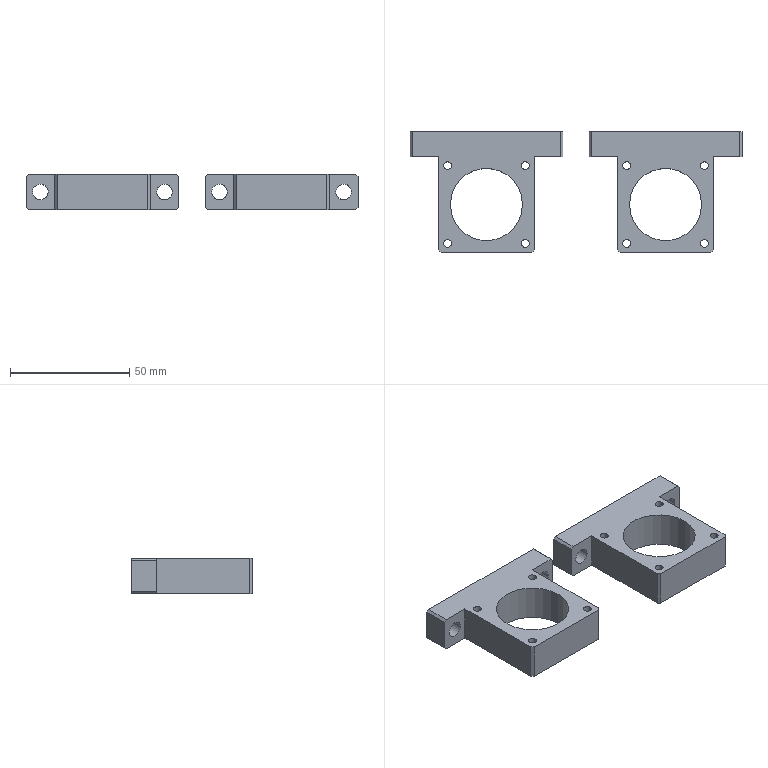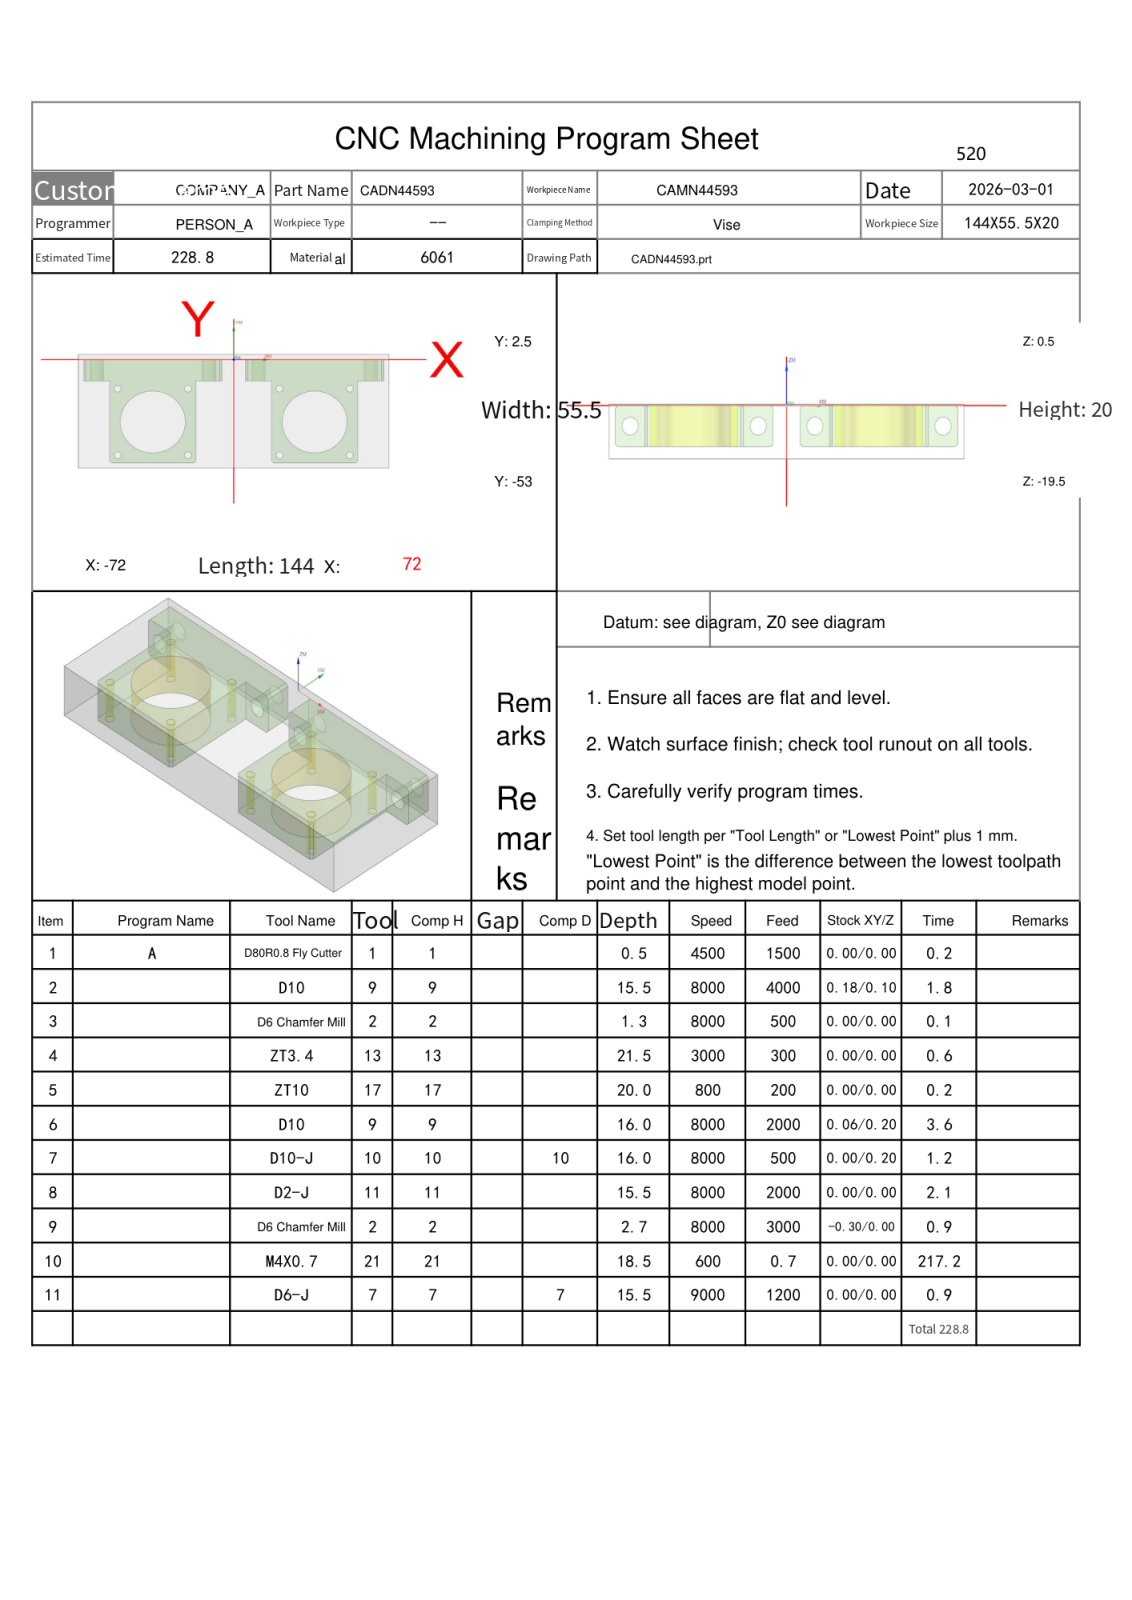NC program | NX | posted by the shop | part box 139 x 50.5 x 15 mm
Lines 2384 to 2729 of 10033:
N3 T02 M06
(D6 Chamfer Mill  D=6. R=0. H=02 ce=0.00 di=0.10)
G00 G90 G54 X21.237 Y-14.237 M03 S8000
G43 H02 Z50.
M08
G98 G81 X21.237 Y-14.237 Z-.8 R1. F500.
X53.763
Y-46.763
X37.5 Y-30.5
X21.237 Y-46.763
X-21.237
Y-14.237
X-37.5 Y-30.5
X-53.763 Y-46.763
Y-14.237
G80
G00 Z50.
G91 G28 Z0.0
M05
M09
G91 G28 Z0.0
M01
N4 T13 M06
(ZT3.4 D=3.4 DR_a=118 H=13)
G00 G90 G54 X-53.763 Y-46.763 M03 S3000
G43 H13 Z50.
M08
G98 G83 X-53.763 Y-46.763 Z-21. R1. F300. Q2.
Y-14.237
X-21.237
Y-46.763
X21.237
X53.763
Y-14.237
X21.237
G80
G00 Z50.
G91 G28 Z0.0
M05
M09
G91 G28 Z0.0
M01
N5 T17 M06
(ZT10 D=10. DR_a=118 H=17)
G00 G90 G54 X-37.5 Y-30.5 M03 S800
G43 H17 Z50.
M08
G98 G83 X-37.5 Y-30.5 Z-19.504 R1. F200. Q2.
X37.5
G80
G00 Z50.
G91 G28 Z0.0
M05
M09
G91 G28 Z0.0
M01
N6 T09 M06
(D10  D=10. R=0. H=09 ce=0.06 di=0.20)
G00 G90 G54 X-37.5 Y-30.5 M03 S8000
G43 H09 Z50.
M08
Z.5
G03 X-35.827 Y-32.173 I1.673 J0.0 F2000.
X-34.153 Y-30.5 I0.0 J1.673
X-34.153 Y-30.5 Z-.1 I-3.347 J0.0
X-34.153 Y-30.5 Z-.7 I-3.347 J0.0
X-34.153 Y-30.5 Z-1.3 I-3.347 J0.0
X-34.153 Y-30.5 Z-1.9 I-3.347 J0.0
X-34.153 Y-30.5 Z-2.5 I-3.347 J0.0
X-34.153 Y-30.5 Z-3.1 I-3.347 J0.0
X-34.153 Y-30.5 Z-3.7 I-3.347 J0.0
X-34.153 Y-30.5 Z-4.3 I-3.347 J0.0
X-34.153 Y-30.5 Z-4.9 I-3.347 J0.0
X-34.153 Y-30.5 Z-5.5 I-3.347 J0.0
X-34.153 Y-30.5 Z-6.1 I-3.347 J0.0
X-34.153 Y-30.5 Z-6.7 I-3.347 J0.0
X-34.153 Y-30.5 Z-7.3 I-3.347 J0.0
X-34.153 Y-30.5 Z-7.9 I-3.347 J0.0
X-34.153 Y-30.5 Z-8.5 I-3.347 J0.0
X-34.153 Y-30.5 Z-9.1 I-3.347 J0.0
X-34.153 Y-30.5 Z-9.7 I-3.347 J0.0
X-34.153 Y-30.5 Z-10.3 I-3.347 J0.0
X-34.153 Y-30.5 Z-10.9 I-3.347 J0.0
X-34.153 Y-30.5 Z-11.5 I-3.347 J0.0
X-34.153 Y-30.5 Z-12.1 I-3.347 J0.0
X-34.153 Y-30.5 Z-12.7 I-3.347 J0.0
X-34.153 Y-30.5 Z-13.3 I-3.347 J0.0
X-34.153 Y-30.5 Z-13.9 I-3.347 J0.0
X-34.153 Y-30.5 Z-14.5 I-3.347 J0.0
X-34.153 Y-30.5 Z-15.1 I-3.347 J0.0
X-39.173 Y-33.398 Z-15.5 I-3.347 J0.0
X-37.5 Y-33.847 I1.673 J2.898
X-34.153 Y-30.5 I0.0 J3.347
X-37.5 Y-27.153 I-3.347 J0.0
X-40.847 Y-30.5 I0.0 J-3.347
X-39.173 Y-33.398 I3.347 J0.0
X-38.337 Y-33.622 I.837 J1.449
X-36.663 Y-31.949 I0.0 J1.673
X-37.5 Y-30.5 I-1.673 J0.0
G00 Z.5
G03 X-34.153 Y-33.847 I3.347 J0.0
X-30.807 Y-30.5 I0.0 J3.347
X-30.807 Y-30.5 Z-.1 I-6.693 J0.0
X-30.807 Y-30.5 Z-.7 I-6.693 J0.0
X-30.807 Y-30.5 Z-1.3 I-6.693 J0.0
X-30.807 Y-30.5 Z-1.9 I-6.693 J0.0
X-30.807 Y-30.5 Z-2.5 I-6.693 J0.0
X-30.807 Y-30.5 Z-3.1 I-6.693 J0.0
X-30.807 Y-30.5 Z-3.7 I-6.693 J0.0
X-30.807 Y-30.5 Z-4.3 I-6.693 J0.0
X-30.807 Y-30.5 Z-4.9 I-6.693 J0.0
X-30.807 Y-30.5 Z-5.5 I-6.693 J0.0
X-30.807 Y-30.5 Z-6.1 I-6.693 J0.0
X-30.807 Y-30.5 Z-6.7 I-6.693 J0.0
X-30.807 Y-30.5 Z-7.3 I-6.693 J0.0
X-30.807 Y-30.5 Z-7.9 I-6.693 J0.0
X-30.807 Y-30.5 Z-8.5 I-6.693 J0.0
X-30.807 Y-30.5 Z-9.1 I-6.693 J0.0
X-30.807 Y-30.5 Z-9.7 I-6.693 J0.0
X-30.807 Y-30.5 Z-10.3 I-6.693 J0.0
X-30.807 Y-30.5 Z-10.9 I-6.693 J0.0
X-30.807 Y-30.5 Z-11.5 I-6.693 J0.0
X-30.807 Y-30.5 Z-12.1 I-6.693 J0.0
X-30.807 Y-30.5 Z-12.7 I-6.693 J0.0
X-30.807 Y-30.5 Z-13.3 I-6.693 J0.0
X-30.807 Y-30.5 Z-13.9 I-6.693 J0.0
X-30.807 Y-30.5 Z-14.5 I-6.693 J0.0
X-30.807 Y-30.5 Z-15.1 I-6.693 J0.0
X-40.847 Y-36.297 Z-15.5 I-6.693 J0.0
X-37.5 Y-37.193 I3.347 J5.797
X-30.807 Y-30.5 I0.0 J6.693
X-37.5 Y-23.807 I-6.693 J0.0
X-44.193 Y-30.5 I0.0 J-6.693
X-40.847 Y-36.297 I6.693 J0.0
X-39.173 Y-36.745 I1.673 J2.898
X-35.827 Y-33.398 I0.0 J3.347
X-37.5 Y-30.5 I-3.347 J0.0
G00 Z.5
G03 X-32.48 Y-35.52 I5.02 J0.0
X-27.46 Y-30.5 I0.0 J5.02
X-27.46 Y-30.5 Z-.1 I-10.04 J0.0
X-27.46 Y-30.5 Z-.7 I-10.04 J0.0
X-27.46 Y-30.5 Z-1.3 I-10.04 J0.0
X-27.46 Y-30.5 Z-1.9 I-10.04 J0.0
X-27.46 Y-30.5 Z-2.5 I-10.04 J0.0
X-27.46 Y-30.5 Z-3.1 I-10.04 J0.0
X-27.46 Y-30.5 Z-3.7 I-10.04 J0.0
X-27.46 Y-30.5 Z-4.3 I-10.04 J0.0
X-27.46 Y-30.5 Z-4.9 I-10.04 J0.0
X-27.46 Y-30.5 Z-5.5 I-10.04 J0.0
X-27.46 Y-30.5 Z-6.1 I-10.04 J0.0
X-27.46 Y-30.5 Z-6.7 I-10.04 J0.0
X-27.46 Y-30.5 Z-7.3 I-10.04 J0.0
X-27.46 Y-30.5 Z-7.9 I-10.04 J0.0
X-27.46 Y-30.5 Z-8.5 I-10.04 J0.0
X-27.46 Y-30.5 Z-9.1 I-10.04 J0.0
X-27.46 Y-30.5 Z-9.7 I-10.04 J0.0
X-27.46 Y-30.5 Z-10.3 I-10.04 J0.0
X-27.46 Y-30.5 Z-10.9 I-10.04 J0.0
X-27.46 Y-30.5 Z-11.5 I-10.04 J0.0
X-27.46 Y-30.5 Z-12.1 I-10.04 J0.0
X-27.46 Y-30.5 Z-12.7 I-10.04 J0.0
X-27.46 Y-30.5 Z-13.3 I-10.04 J0.0
X-27.46 Y-30.5 Z-13.9 I-10.04 J0.0
X-27.46 Y-30.5 Z-14.5 I-10.04 J0.0
X-27.46 Y-30.5 Z-15.1 I-10.04 J0.0
X-42.52 Y-39.195 Z-15.5 I-10.04 J0.0
X-37.5 Y-40.54 I5.02 J8.695
X-27.46 Y-30.5 I0.0 J10.04
X-37.5 Y-20.46 I-10.04 J0.0
X-47.54 Y-30.5 I0.0 J-10.04
X-42.52 Y-39.195 I10.04 J0.0
X-40.01 Y-39.867 I2.51 J4.347
X-34.99 Y-34.847 I0.0 J5.02
X-37.5 Y-30.5 I-5.02 J0.0
G00 Z50.
X37.5
Z.5
G03 X39.173 Y-32.173 I1.673 J0.0
X40.847 Y-30.5 I0.0 J1.673
X40.847 Y-30.5 Z-.1 I-3.347 J0.0
X40.847 Y-30.5 Z-.7 I-3.347 J0.0
X40.847 Y-30.5 Z-1.3 I-3.347 J0.0
X40.847 Y-30.5 Z-1.9 I-3.347 J0.0
X40.847 Y-30.5 Z-2.5 I-3.347 J0.0
X40.847 Y-30.5 Z-3.1 I-3.347 J0.0
X40.847 Y-30.5 Z-3.7 I-3.347 J0.0
X40.847 Y-30.5 Z-4.3 I-3.347 J0.0
X40.847 Y-30.5 Z-4.9 I-3.347 J0.0
X40.847 Y-30.5 Z-5.5 I-3.347 J0.0
X40.847 Y-30.5 Z-6.1 I-3.347 J0.0
X40.847 Y-30.5 Z-6.7 I-3.347 J0.0
X40.847 Y-30.5 Z-7.3 I-3.347 J0.0
X40.847 Y-30.5 Z-7.9 I-3.347 J0.0
X40.847 Y-30.5 Z-8.5 I-3.347 J0.0
X40.847 Y-30.5 Z-9.1 I-3.347 J0.0
X40.847 Y-30.5 Z-9.7 I-3.347 J0.0
X40.847 Y-30.5 Z-10.3 I-3.347 J0.0
X40.847 Y-30.5 Z-10.9 I-3.347 J0.0
X40.847 Y-30.5 Z-11.5 I-3.347 J0.0
X40.847 Y-30.5 Z-12.1 I-3.347 J0.0
X40.847 Y-30.5 Z-12.7 I-3.347 J0.0
X40.847 Y-30.5 Z-13.3 I-3.347 J0.0
X40.847 Y-30.5 Z-13.9 I-3.347 J0.0
X40.847 Y-30.5 Z-14.5 I-3.347 J0.0
X40.847 Y-30.5 Z-15.1 I-3.347 J0.0
X35.827 Y-33.398 Z-15.5 I-3.347 J0.0
X37.5 Y-33.847 I1.673 J2.898
X40.847 Y-30.5 I0.0 J3.347
X37.5 Y-27.153 I-3.347 J0.0
X34.153 Y-30.5 I0.0 J-3.347
X35.827 Y-33.398 I3.347 J0.0
X36.663 Y-33.622 I.837 J1.449
X38.337 Y-31.949 I0.0 J1.673
X37.5 Y-30.5 I-1.673 J0.0
G00 Z.5
G03 X40.847 Y-33.847 I3.347 J0.0
X44.193 Y-30.5 I0.0 J3.347
X44.193 Y-30.5 Z-.1 I-6.693 J0.0
X44.193 Y-30.5 Z-.7 I-6.693 J0.0
X44.193 Y-30.5 Z-1.3 I-6.693 J0.0
X44.193 Y-30.5 Z-1.9 I-6.693 J0.0
X44.193 Y-30.5 Z-2.5 I-6.693 J0.0
X44.193 Y-30.5 Z-3.1 I-6.693 J0.0
X44.193 Y-30.5 Z-3.7 I-6.693 J0.0
X44.193 Y-30.5 Z-4.3 I-6.693 J0.0
X44.193 Y-30.5 Z-4.9 I-6.693 J0.0
X44.193 Y-30.5 Z-5.5 I-6.693 J0.0
X44.193 Y-30.5 Z-6.1 I-6.693 J0.0
X44.193 Y-30.5 Z-6.7 I-6.693 J0.0
X44.193 Y-30.5 Z-7.3 I-6.693 J0.0
X44.193 Y-30.5 Z-7.9 I-6.693 J0.0
X44.193 Y-30.5 Z-8.5 I-6.693 J0.0
X44.193 Y-30.5 Z-9.1 I-6.693 J0.0
X44.193 Y-30.5 Z-9.7 I-6.693 J0.0
X44.193 Y-30.5 Z-10.3 I-6.693 J0.0
X44.193 Y-30.5 Z-10.9 I-6.693 J0.0
X44.193 Y-30.5 Z-11.5 I-6.693 J0.0
X44.193 Y-30.5 Z-12.1 I-6.693 J0.0
X44.193 Y-30.5 Z-12.7 I-6.693 J0.0
X44.193 Y-30.5 Z-13.3 I-6.693 J0.0
X44.193 Y-30.5 Z-13.9 I-6.693 J0.0
X44.193 Y-30.5 Z-14.5 I-6.693 J0.0
X44.193 Y-30.5 Z-15.1 I-6.693 J0.0
X34.153 Y-36.297 Z-15.5 I-6.693 J0.0
X37.5 Y-37.193 I3.347 J5.797
X44.193 Y-30.5 I0.0 J6.693
X37.5 Y-23.807 I-6.693 J0.0
X30.807 Y-30.5 I0.0 J-6.693
X34.153 Y-36.297 I6.693 J0.0
X35.827 Y-36.745 I1.673 J2.898
X39.173 Y-33.398 I0.0 J3.347
X37.5 Y-30.5 I-3.347 J0.0
G00 Z.5
G03 X42.52 Y-35.52 I5.02 J0.0
X47.54 Y-30.5 I0.0 J5.02
X47.54 Y-30.5 Z-.1 I-10.04 J0.0
X47.54 Y-30.5 Z-.7 I-10.04 J0.0
X47.54 Y-30.5 Z-1.3 I-10.04 J0.0
X47.54 Y-30.5 Z-1.9 I-10.04 J0.0
X47.54 Y-30.5 Z-2.5 I-10.04 J0.0
X47.54 Y-30.5 Z-3.1 I-10.04 J0.0
X47.54 Y-30.5 Z-3.7 I-10.04 J0.0
X47.54 Y-30.5 Z-4.3 I-10.04 J0.0
X47.54 Y-30.5 Z-4.9 I-10.04 J0.0
X47.54 Y-30.5 Z-5.5 I-10.04 J0.0
X47.54 Y-30.5 Z-6.1 I-10.04 J0.0
X47.54 Y-30.5 Z-6.7 I-10.04 J0.0
X47.54 Y-30.5 Z-7.3 I-10.04 J0.0
X47.54 Y-30.5 Z-7.9 I-10.04 J0.0
X47.54 Y-30.5 Z-8.5 I-10.04 J0.0
X47.54 Y-30.5 Z-9.1 I-10.04 J0.0
X47.54 Y-30.5 Z-9.7 I-10.04 J0.0
X47.54 Y-30.5 Z-10.3 I-10.04 J0.0
X47.54 Y-30.5 Z-10.9 I-10.04 J0.0
X47.54 Y-30.5 Z-11.5 I-10.04 J0.0
X47.54 Y-30.5 Z-12.1 I-10.04 J0.0
X47.54 Y-30.5 Z-12.7 I-10.04 J0.0
X47.54 Y-30.5 Z-13.3 I-10.04 J0.0
X47.54 Y-30.5 Z-13.9 I-10.04 J0.0
X47.54 Y-30.5 Z-14.5 I-10.04 J0.0
X47.54 Y-30.5 Z-15.1 I-10.04 J0.0
X32.48 Y-39.195 Z-15.5 I-10.04 J0.0
X37.5 Y-40.54 I5.02 J8.695
X47.54 Y-30.5 I0.0 J10.04
X37.5 Y-20.46 I-10.04 J0.0
X27.46 Y-30.5 I0.0 J-10.04
X32.48 Y-39.195 I10.04 J0.0
X34.99 Y-39.867 I2.51 J4.347
X40.01 Y-34.847 I0.0 J5.02
X37.5 Y-30.5 I-5.02 J0.0
G00 Z50.
G91 G28 Z0.0
M05
M09
G91 G28 Z0.0
M01
N7 T10 M06
(D10-J  D=10. R=0. H=10 ce=0.00 di=0.20)
G00 G90 G54 X-37.5 Y-30.5 M03 S8000
G43 H10 Z50.
M08
Z.5
G41 D10
G01 X-30.895 Y-32.936 F500.
G03 X-29.996 Y-33.096 I.898 J2.436
X-27.4 Y-30.5 I0.0 J2.596
X-27.4 Y-30.5 Z-4.5 I-10.1 J0.0
X-27.4 Y-30.5 Z-9.5 I-10.1 J0.0
X-27.4 Y-30.5 Z-14.5 I-10.1 J0.0
X-34.379 Y-20.894 Z-15.5 I-10.1 J0.0
X-37.5 Y-20.4 I-3.121 J-9.606
X-47.6 Y-30.5 I0.0 J-10.1
X-37.5 Y-40.6 I10.1 J0.0
X-27.4 Y-30.5 I0.0 J10.1
X-34.379 Y-20.894 I-10.1 J0.0
X-35.181 Y-20.767 I-.802 J-2.469
X-37.778 Y-23.364 I0.0 J-2.596
G01 X-37.776 Y-23.465
G40 X-37.5 Y-30.5
G00 Z50.
X37.5
Z.5
G41 D10
G01 X44.105 Y-32.936
G03 X45.004 Y-33.096 I.898 J2.436
X47.6 Y-30.5 I0.0 J2.596
X47.6 Y-30.5 Z-4.5 I-10.1 J0.0
X47.6 Y-30.5 Z-9.5 I-10.1 J0.0
X47.6 Y-30.5 Z-14.5 I-10.1 J0.0
X40.621 Y-20.894 Z-15.5 I-10.1 J0.0
X37.5 Y-20.4 I-3.121 J-9.606
X27.4 Y-30.5 I0.0 J-10.1
X37.5 Y-40.6 I10.1 J0.0
X47.6 Y-30.5 I0.0 J10.1
X40.621 Y-20.894 I-10.1 J0.0
X39.819 Y-20.767 I-.802 J-2.469
X37.222 Y-23.364 I0.0 J-2.596
G01 X37.224 Y-23.465
G40 X37.5 Y-30.5
G00 Z50.
G91 G28 Z0.0
M05
M09
G91 G28 Z0.0
M01